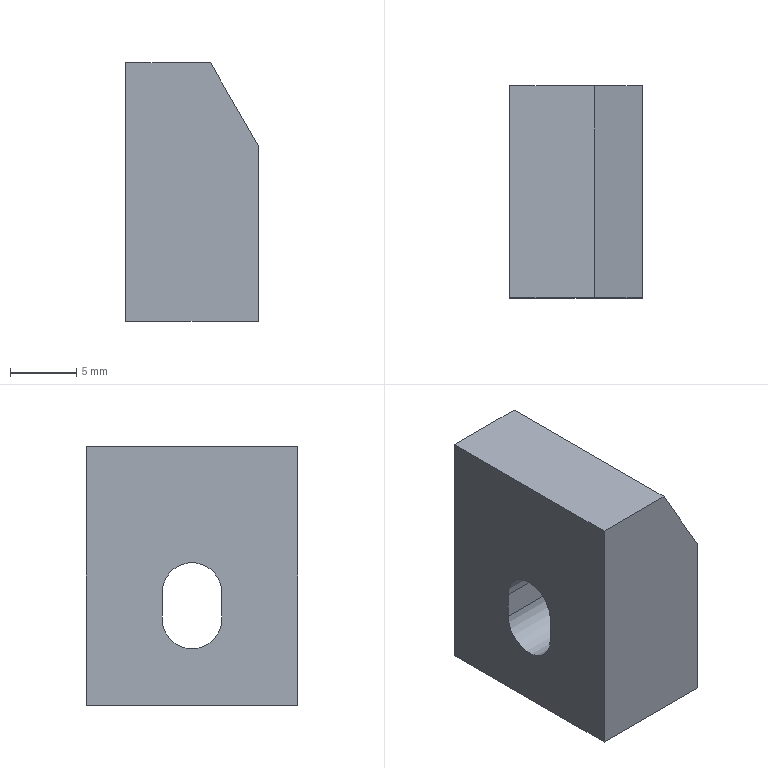Part | STEP file | 4-20.sldasm-Part-196 | 1 solid | 16 faces | box 10 x 16 x 19.5 mm | volume 2443 mm3 | plane 12 | cylinder 4 | commonest cylinder face diameters 4.5 x2 8 x2
STEP:
#1=CARTESIAN_POINT('',(132.065,605.425,-80.993));
#2=VERTEX_POINT('',#1);
#3=CARTESIAN_POINT('',(132.065,605.425,-100.493));
#4=VERTEX_POINT('',#3);
#5=CARTESIAN_POINT('',(132.065,605.425,-73.493));
#6=DIRECTION('',(0.,0.,-1.));
#7=VECTOR('',#6,1000.);
#8=LINE('',#5,#7);
#9=EDGE_CURVE('',#2,#4,#8,.T.);
#10=ORIENTED_EDGE('',*,*,#9,.T.);
#11=CARTESIAN_POINT('',(132.065,589.425,-100.493));
#12=VERTEX_POINT('',#11);
#13=CARTESIAN_POINT('',(132.065,589.425,-100.493));
#14=DIRECTION('',(0.,1.,0.));
#15=VECTOR('',#14,1000.);
#16=LINE('',#13,#15);
#17=EDGE_CURVE('',#12,#4,#16,.T.);
#18=ORIENTED_EDGE('',*,*,#17,.F.);
#19=CARTESIAN_POINT('',(132.065,589.425,-80.993));
#20=VERTEX_POINT('',#19);
#21=CARTESIAN_POINT('',(132.065,589.425,-73.493));
#22=DIRECTION('',(0.,0.,-1.));
#23=VECTOR('',#22,1000.);
#24=LINE('',#21,#23);
#25=EDGE_CURVE('',#20,#12,#24,.T.);
#26=ORIENTED_EDGE('',*,*,#25,.F.);
#27=CARTESIAN_POINT('',(132.065,1166.425,-80.993));
#28=DIRECTION('',(0.,1.,0.));
#29=VECTOR('',#28,1000.);
#30=LINE('',#27,#29);
#31=EDGE_CURVE('',#20,#2,#30,.T.);
#32=ORIENTED_EDGE('',*,*,#31,.T.);
#33=EDGE_LOOP('',(#10,#18,#26,#32));
#34=FACE_OUTER_BOUND('',#33,.T.);
#35=CARTESIAN_POINT('',(132.065,599.675,-93.993));
#36=VERTEX_POINT('',#35);
#37=CARTESIAN_POINT('',(132.065,595.175,-93.993));
#38=VERTEX_POINT('',#37);
#39=CARTESIAN_POINT('',(132.065,597.425,-93.993));
#40=DIRECTION('',(-1.,0.,0.));
#41=DIRECTION('',(0.,-1.,0.));
#42=AXIS2_PLACEMENT_3D('',#39,#40,#41);
#43=CIRCLE('',#42,2.25);
#44=EDGE_CURVE('',#36,#38,#43,.T.);
#45=ORIENTED_EDGE('',*,*,#44,.F.);
#46=CARTESIAN_POINT('',(132.065,599.675,-91.993));
#47=VERTEX_POINT('',#46);
#48=CARTESIAN_POINT('',(132.065,599.675,-73.493));
#49=DIRECTION('',(0.,0.,1.));
#50=VECTOR('',#49,1000.);
#51=LINE('',#48,#50);
#52=EDGE_CURVE('',#36,#47,#51,.T.);
#53=ORIENTED_EDGE('',*,*,#52,.T.);
#54=CARTESIAN_POINT('',(132.065,595.175,-91.993));
#55=VERTEX_POINT('',#54);
#56=CARTESIAN_POINT('',(132.065,597.425,-91.993));
#57=DIRECTION('',(-1.,0.,0.));
#58=DIRECTION('',(0.,-1.,0.));
#59=AXIS2_PLACEMENT_3D('',#56,#57,#58);
#60=CIRCLE('',#59,2.25);
#61=EDGE_CURVE('',#55,#47,#60,.T.);
#62=ORIENTED_EDGE('',*,*,#61,.F.);
#63=CARTESIAN_POINT('',(132.065,595.175,-73.493));
#64=DIRECTION('',(0.,0.,-1.));
#65=VECTOR('',#64,1000.);
#66=LINE('',#63,#65);
#67=EDGE_CURVE('',#55,#38,#66,.T.);
#68=ORIENTED_EDGE('',*,*,#67,.T.);
#69=EDGE_LOOP('',(#45,#53,#62,#68));
#70=FACE_BOUND('',#69,.T.);
#71=CARTESIAN_POINT('',(132.065,589.425,-73.493));
#72=DIRECTION('',(1.,0.,0.));
#73=DIRECTION('',(0.,-1.,0.));
#74=AXIS2_PLACEMENT_3D('',#71,#72,#73);
#75=PLANE('',#74);
#76=ADVANCED_FACE('',(#34,#70),#75,.F.);
#77=CARTESIAN_POINT('',(136.065,593.425,-93.993));
#78=VERTEX_POINT('',#77);
#79=CARTESIAN_POINT('',(136.065,601.425,-93.993));
#80=VERTEX_POINT('',#79);
#81=CARTESIAN_POINT('',(136.065,597.425,-93.993));
#82=DIRECTION('',(1.,0.,0.));
#83=DIRECTION('',(0.,-1.,0.));
#84=AXIS2_PLACEMENT_3D('',#81,#82,#83);
#85=CIRCLE('',#84,4.);
#86=EDGE_CURVE('',#78,#80,#85,.T.);
#87=ORIENTED_EDGE('',*,*,#86,.T.);
#88=CARTESIAN_POINT('',(136.065,601.425,-91.993));
#89=VERTEX_POINT('',#88);
#90=CARTESIAN_POINT('',(136.065,601.425,-97.993));
#91=DIRECTION('',(0.,0.,1.));
#92=VECTOR('',#91,1000.);
#93=LINE('',#90,#92);
#94=EDGE_CURVE('',#80,#89,#93,.T.);
#95=ORIENTED_EDGE('',*,*,#94,.T.);
#96=CARTESIAN_POINT('',(136.065,593.425,-91.993));
#97=VERTEX_POINT('',#96);
#98=CARTESIAN_POINT('',(136.065,597.425,-91.993));
#99=DIRECTION('',(1.,0.,0.));
#100=DIRECTION('',(0.,-1.,0.));
#101=AXIS2_PLACEMENT_3D('',#98,#99,#100);
#102=CIRCLE('',#101,4.);
#103=EDGE_CURVE('',#89,#97,#102,.T.);
#104=ORIENTED_EDGE('',*,*,#103,.T.);
#105=CARTESIAN_POINT('',(136.065,593.425,-97.993));
#106=DIRECTION('',(0.,0.,1.));
#107=VECTOR('',#106,1000.);
#108=LINE('',#105,#107);
#109=EDGE_CURVE('',#78,#97,#108,.T.);
#110=ORIENTED_EDGE('',*,*,#109,.F.);
#111=EDGE_LOOP('',(#87,#95,#104,#110));
#112=FACE_OUTER_BOUND('',#111,.T.);
#113=CARTESIAN_POINT('',(136.065,599.675,-93.993));
#114=VERTEX_POINT('',#113);
#115=CARTESIAN_POINT('',(136.065,599.675,-91.993));
#116=VERTEX_POINT('',#115);
#117=CARTESIAN_POINT('',(136.065,599.675,-97.993));
#118=DIRECTION('',(0.,0.,1.));
#119=VECTOR('',#118,1000.);
#120=LINE('',#117,#119);
#121=EDGE_CURVE('',#114,#116,#120,.T.);
#122=ORIENTED_EDGE('',*,*,#121,.F.);
#123=CARTESIAN_POINT('',(136.065,595.175,-93.993));
#124=VERTEX_POINT('',#123);
#125=CARTESIAN_POINT('',(136.065,597.425,-93.993));
#126=DIRECTION('',(-1.,0.,0.));
#127=DIRECTION('',(0.,-1.,0.));
#128=AXIS2_PLACEMENT_3D('',#125,#126,#127);
#129=CIRCLE('',#128,2.25);
#130=EDGE_CURVE('',#114,#124,#129,.T.);
#131=ORIENTED_EDGE('',*,*,#130,.T.);
#132=CARTESIAN_POINT('',(136.065,595.175,-91.993));
#133=VERTEX_POINT('',#132);
#134=CARTESIAN_POINT('',(136.065,595.175,-97.993));
#135=DIRECTION('',(0.,0.,-1.));
#136=VECTOR('',#135,1000.);
#137=LINE('',#134,#136);
#138=EDGE_CURVE('',#133,#124,#137,.T.);
#139=ORIENTED_EDGE('',*,*,#138,.F.);
#140=CARTESIAN_POINT('',(136.065,597.425,-91.993));
#141=DIRECTION('',(-1.,0.,0.));
#142=DIRECTION('',(0.,-1.,0.));
#143=AXIS2_PLACEMENT_3D('',#140,#141,#142);
#144=CIRCLE('',#143,2.25);
#145=EDGE_CURVE('',#133,#116,#144,.T.);
#146=ORIENTED_EDGE('',*,*,#145,.T.);
#147=EDGE_LOOP('',(#122,#131,#139,#146));
#148=FACE_BOUND('',#147,.T.);
#149=CARTESIAN_POINT('',(136.065,597.425,-97.993));
#150=DIRECTION('',(1.,0.,0.));
#151=DIRECTION('',(0.,-1.,0.));
#152=AXIS2_PLACEMENT_3D('',#149,#150,#151);
#153=PLANE('',#152);
#154=ADVANCED_FACE('',(#112,#148),#153,.T.);
#155=CARTESIAN_POINT('',(142.065,605.425,-100.493));
#156=VERTEX_POINT('',#155);
#157=CARTESIAN_POINT('',(142.065,605.425,-87.23));
#158=VERTEX_POINT('',#157);
#159=CARTESIAN_POINT('',(142.065,605.425,-103.493));
#160=DIRECTION('',(0.,0.,1.));
#161=VECTOR('',#160,1000.);
#162=LINE('',#159,#161);
#163=EDGE_CURVE('',#156,#158,#162,.T.);
#164=ORIENTED_EDGE('',*,*,#163,.T.);
#165=CARTESIAN_POINT('',(142.065,589.425,-87.23));
#166=VERTEX_POINT('',#165);
#167=CARTESIAN_POINT('',(142.065,605.425,-87.23));
#168=DIRECTION('',(0.,1.,0.));
#169=VECTOR('',#168,1000.);
#170=LINE('',#167,#169);
#171=EDGE_CURVE('',#166,#158,#170,.T.);
#172=ORIENTED_EDGE('',*,*,#171,.F.);
#173=CARTESIAN_POINT('',(142.065,589.425,-100.493));
#174=VERTEX_POINT('',#173);
#175=CARTESIAN_POINT('',(142.065,589.425,-103.493));
#176=DIRECTION('',(0.,0.,1.));
#177=VECTOR('',#176,1000.);
#178=LINE('',#175,#177);
#179=EDGE_CURVE('',#174,#166,#178,.T.);
#180=ORIENTED_EDGE('',*,*,#179,.F.);
#181=CARTESIAN_POINT('',(142.065,1211.425,-100.493));
#182=DIRECTION('',(0.,1.,0.));
#183=VECTOR('',#182,1000.);
#184=LINE('',#181,#183);
#185=EDGE_CURVE('',#174,#156,#184,.T.);
#186=ORIENTED_EDGE('',*,*,#185,.T.);
#187=EDGE_LOOP('',(#164,#172,#180,#186));
#188=FACE_OUTER_BOUND('',#187,.T.);
#189=CARTESIAN_POINT('',(142.065,593.425,-93.993));
#190=VERTEX_POINT('',#189);
#191=CARTESIAN_POINT('',(142.065,601.425,-93.993));
#192=VERTEX_POINT('',#191);
#193=CARTESIAN_POINT('',(142.065,597.425,-93.993));
#194=DIRECTION('',(1.,0.,0.));
#195=DIRECTION('',(0.,0.,-1.));
#196=AXIS2_PLACEMENT_3D('',#193,#194,#195);
#197=CIRCLE('',#196,4.);
#198=EDGE_CURVE('',#190,#192,#197,.T.);
#199=ORIENTED_EDGE('',*,*,#198,.F.);
#200=CARTESIAN_POINT('',(142.065,593.425,-91.993));
#201=VERTEX_POINT('',#200);
#202=CARTESIAN_POINT('',(142.065,593.425,-103.493));
#203=DIRECTION('',(0.,0.,1.));
#204=VECTOR('',#203,1000.);
#205=LINE('',#202,#204);
#206=EDGE_CURVE('',#190,#201,#205,.T.);
#207=ORIENTED_EDGE('',*,*,#206,.T.);
#208=CARTESIAN_POINT('',(142.065,601.425,-91.993));
#209=VERTEX_POINT('',#208);
#210=CARTESIAN_POINT('',(142.065,597.425,-91.993));
#211=DIRECTION('',(1.,0.,0.));
#212=DIRECTION('',(0.,0.,-1.));
#213=AXIS2_PLACEMENT_3D('',#210,#211,#212);
#214=CIRCLE('',#213,4.);
#215=EDGE_CURVE('',#209,#201,#214,.T.);
#216=ORIENTED_EDGE('',*,*,#215,.F.);
#217=CARTESIAN_POINT('',(142.065,601.425,-103.493));
#218=DIRECTION('',(0.,0.,1.));
#219=VECTOR('',#218,1000.);
#220=LINE('',#217,#219);
#221=EDGE_CURVE('',#192,#209,#220,.T.);
#222=ORIENTED_EDGE('',*,*,#221,.F.);
#223=EDGE_LOOP('',(#199,#207,#216,#222));
#224=FACE_BOUND('',#223,.T.);
#225=CARTESIAN_POINT('',(142.065,589.425,-103.493));
#226=DIRECTION('',(-1.,0.,0.));
#227=DIRECTION('',(0.,0.,-1.));
#228=AXIS2_PLACEMENT_3D('',#225,#226,#227);
#229=PLANE('',#228);
#230=ADVANCED_FACE('',(#188,#224),#229,.F.);
#231=CARTESIAN_POINT('',(132.065,605.425,-100.493));
#232=DIRECTION('',(1.,0.,0.));
#233=VECTOR('',#232,1000.);
#234=LINE('',#231,#233);
#235=EDGE_CURVE('',#4,#156,#234,.T.);
#236=ORIENTED_EDGE('',*,*,#235,.T.);
#237=ORIENTED_EDGE('',*,*,#185,.F.);
#238=CARTESIAN_POINT('',(132.065,589.425,-100.493));
#239=DIRECTION('',(1.,0.,0.));
#240=VECTOR('',#239,1000.);
#241=LINE('',#238,#240);
#242=EDGE_CURVE('',#12,#174,#241,.T.);
#243=ORIENTED_EDGE('',*,*,#242,.F.);
#244=ORIENTED_EDGE('',*,*,#17,.T.);
#245=EDGE_LOOP('',(#236,#237,#243,#244));
#246=FACE_OUTER_BOUND('',#245,.T.);
#247=CARTESIAN_POINT('',(-227.636,1211.425,-100.493));
#248=DIRECTION('',(0.,0.,-1.));
#249=DIRECTION('',(1.,0.,0.));
#250=AXIS2_PLACEMENT_3D('',#247,#248,#249);
#251=PLANE('',#250);
#252=ADVANCED_FACE('',(#246),#251,.T.);
#253=CARTESIAN_POINT('',(138.464,605.425,-80.993));
#254=VERTEX_POINT('',#253);
#255=CARTESIAN_POINT('',(142.065,605.425,-87.23));
#256=DIRECTION('',(-0.5,0.,0.866));
#257=VECTOR('',#256,1000.);
#258=LINE('',#255,#257);
#259=EDGE_CURVE('',#158,#254,#258,.T.);
#260=ORIENTED_EDGE('',*,*,#259,.T.);
#261=CARTESIAN_POINT('',(138.464,589.425,-80.993));
#262=VERTEX_POINT('',#261);
#263=CARTESIAN_POINT('',(138.464,605.425,-80.993));
#264=DIRECTION('',(0.,1.,0.));
#265=VECTOR('',#264,1000.);
#266=LINE('',#263,#265);
#267=EDGE_CURVE('',#262,#254,#266,.T.);
#268=ORIENTED_EDGE('',*,*,#267,.F.);
#269=CARTESIAN_POINT('',(142.065,589.425,-87.23));
#270=DIRECTION('',(-0.5,0.,0.866));
#271=VECTOR('',#270,1000.);
#272=LINE('',#269,#271);
#273=EDGE_CURVE('',#166,#262,#272,.T.);
#274=ORIENTED_EDGE('',*,*,#273,.F.);
#275=ORIENTED_EDGE('',*,*,#171,.T.);
#276=EDGE_LOOP('',(#260,#268,#274,#275));
#277=FACE_OUTER_BOUND('',#276,.T.);
#278=CARTESIAN_POINT('',(142.065,605.425,-87.23));
#279=DIRECTION('',(0.866,0.,0.5));
#280=DIRECTION('',(0.5,0.,-0.866));
#281=AXIS2_PLACEMENT_3D('',#278,#279,#280);
#282=PLANE('',#281);
#283=ADVANCED_FACE('',(#277),#282,.T.);
#284=CARTESIAN_POINT('',(132.065,605.425,-80.993));
#285=DIRECTION('',(-1.,0.,0.));
#286=VECTOR('',#285,1000.);
#287=LINE('',#284,#286);
#288=EDGE_CURVE('',#254,#2,#287,.T.);
#289=ORIENTED_EDGE('',*,*,#288,.T.);
#290=ORIENTED_EDGE('',*,*,#31,.F.);
#291=CARTESIAN_POINT('',(132.065,589.425,-80.993));
#292=DIRECTION('',(-1.,0.,0.));
#293=VECTOR('',#292,1000.);
#294=LINE('',#291,#293);
#295=EDGE_CURVE('',#262,#20,#294,.T.);
#296=ORIENTED_EDGE('',*,*,#295,.F.);
#297=ORIENTED_EDGE('',*,*,#267,.T.);
#298=EDGE_LOOP('',(#289,#290,#296,#297));
#299=FACE_OUTER_BOUND('',#298,.T.);
#300=CARTESIAN_POINT('',(152.993,1166.425,-80.993));
#301=DIRECTION('',(0.,0.,-1.));
#302=DIRECTION('',(-1.,0.,0.));
#303=AXIS2_PLACEMENT_3D('',#300,#301,#302);
#304=PLANE('',#303);
#305=ADVANCED_FACE('',(#299),#304,.F.);
#306=ORIENTED_EDGE('',*,*,#25,.T.);
#307=ORIENTED_EDGE('',*,*,#242,.T.);
#308=ORIENTED_EDGE('',*,*,#179,.T.);
#309=ORIENTED_EDGE('',*,*,#273,.T.);
#310=ORIENTED_EDGE('',*,*,#295,.T.);
#311=EDGE_LOOP('',(#306,#307,#308,#309,#310));
#312=FACE_OUTER_BOUND('',#311,.T.);
#313=CARTESIAN_POINT('',(132.065,589.425,-103.493));
#314=DIRECTION('',(0.,-1.,0.));
#315=DIRECTION('',(-1.,0.,0.));
#316=AXIS2_PLACEMENT_3D('',#313,#314,#315);
#317=PLANE('',#316);
#318=ADVANCED_FACE('',(#312),#317,.T.);
#319=ORIENTED_EDGE('',*,*,#9,.F.);
#320=ORIENTED_EDGE('',*,*,#288,.F.);
#321=ORIENTED_EDGE('',*,*,#259,.F.);
#322=ORIENTED_EDGE('',*,*,#163,.F.);
#323=ORIENTED_EDGE('',*,*,#235,.F.);
#324=EDGE_LOOP('',(#319,#320,#321,#322,#323));
#325=FACE_OUTER_BOUND('',#324,.T.);
#326=CARTESIAN_POINT('',(132.065,605.425,-103.493));
#327=DIRECTION('',(0.,-1.,0.));
#328=DIRECTION('',(-1.,0.,0.));
#329=AXIS2_PLACEMENT_3D('',#326,#327,#328);
#330=PLANE('',#329);
#331=ADVANCED_FACE('',(#325),#330,.F.);
#332=ORIENTED_EDGE('',*,*,#198,.T.);
#333=CARTESIAN_POINT('',(145.065,601.425,-93.993));
#334=DIRECTION('',(-1.,0.,0.));
#335=VECTOR('',#334,1000.);
#336=LINE('',#333,#335);
#337=EDGE_CURVE('',#192,#80,#336,.T.);
#338=ORIENTED_EDGE('',*,*,#337,.T.);
#339=ORIENTED_EDGE('',*,*,#86,.F.);
#340=CARTESIAN_POINT('',(145.065,593.425,-93.993));
#341=DIRECTION('',(-1.,0.,0.));
#342=VECTOR('',#341,1000.);
#343=LINE('',#340,#342);
#344=EDGE_CURVE('',#190,#78,#343,.T.);
#345=ORIENTED_EDGE('',*,*,#344,.F.);
#346=EDGE_LOOP('',(#332,#338,#339,#345));
#347=FACE_OUTER_BOUND('',#346,.T.);
#348=CARTESIAN_POINT('',(145.065,597.425,-93.993));
#349=DIRECTION('',(-1.,0.,0.));
#350=DIRECTION('',(0.,1.,0.));
#351=AXIS2_PLACEMENT_3D('',#348,#349,#350);
#352=CYLINDRICAL_SURFACE('',#351,4.);
#353=ADVANCED_FACE('',(#347),#352,.F.);
#354=ORIENTED_EDGE('',*,*,#221,.T.);
#355=CARTESIAN_POINT('',(145.065,601.425,-91.993));
#356=DIRECTION('',(-1.,0.,0.));
#357=VECTOR('',#356,1000.);
#358=LINE('',#355,#357);
#359=EDGE_CURVE('',#209,#89,#358,.T.);
#360=ORIENTED_EDGE('',*,*,#359,.T.);
#361=ORIENTED_EDGE('',*,*,#94,.F.);
#362=ORIENTED_EDGE('',*,*,#337,.F.);
#363=EDGE_LOOP('',(#354,#360,#361,#362));
#364=FACE_OUTER_BOUND('',#363,.T.);
#365=CARTESIAN_POINT('',(145.065,601.425,-97.993));
#366=DIRECTION('',(0.,-1.,0.));
#367=DIRECTION('',(-1.,0.,0.));
#368=AXIS2_PLACEMENT_3D('',#365,#366,#367);
#369=PLANE('',#368);
#370=ADVANCED_FACE('',(#364),#369,.T.);
#371=ORIENTED_EDGE('',*,*,#215,.T.);
#372=CARTESIAN_POINT('',(145.065,593.425,-91.993));
#373=DIRECTION('',(-1.,0.,0.));
#374=VECTOR('',#373,1000.);
#375=LINE('',#372,#374);
#376=EDGE_CURVE('',#201,#97,#375,.T.);
#377=ORIENTED_EDGE('',*,*,#376,.T.);
#378=ORIENTED_EDGE('',*,*,#103,.F.);
#379=ORIENTED_EDGE('',*,*,#359,.F.);
#380=EDGE_LOOP('',(#371,#377,#378,#379));
#381=FACE_OUTER_BOUND('',#380,.T.);
#382=CARTESIAN_POINT('',(145.065,597.425,-91.993));
#383=DIRECTION('',(-1.,0.,0.));
#384=DIRECTION('',(0.,1.,0.));
#385=AXIS2_PLACEMENT_3D('',#382,#383,#384);
#386=CYLINDRICAL_SURFACE('',#385,4.);
#387=ADVANCED_FACE('',(#381),#386,.F.);
#388=ORIENTED_EDGE('',*,*,#344,.T.);
#389=ORIENTED_EDGE('',*,*,#109,.T.);
#390=ORIENTED_EDGE('',*,*,#376,.F.);
#391=ORIENTED_EDGE('',*,*,#206,.F.);
#392=EDGE_LOOP('',(#388,#389,#390,#391));
#393=FACE_OUTER_BOUND('',#392,.T.);
#394=CARTESIAN_POINT('',(145.065,593.425,-97.993));
#395=DIRECTION('',(0.,-1.,0.));
#396=DIRECTION('',(-1.,0.,0.));
#397=AXIS2_PLACEMENT_3D('',#394,#395,#396);
#398=PLANE('',#397);
#399=ADVANCED_FACE('',(#393),#398,.F.);
#400=ORIENTED_EDGE('',*,*,#44,.T.);
#401=CARTESIAN_POINT('',(145.065,595.175,-93.993));
#402=DIRECTION('',(-1.,0.,0.));
#403=VECTOR('',#402,1000.);
#404=LINE('',#401,#403);
#405=EDGE_CURVE('',#124,#38,#404,.T.);
#406=ORIENTED_EDGE('',*,*,#405,.F.);
#407=ORIENTED_EDGE('',*,*,#130,.F.);
#408=CARTESIAN_POINT('',(145.065,599.675,-93.993));
#409=DIRECTION('',(-1.,0.,0.));
#410=VECTOR('',#409,1000.);
#411=LINE('',#408,#410);
#412=EDGE_CURVE('',#114,#36,#411,.T.);
#413=ORIENTED_EDGE('',*,*,#412,.T.);
#414=EDGE_LOOP('',(#400,#406,#407,#413));
#415=FACE_OUTER_BOUND('',#414,.T.);
#416=CARTESIAN_POINT('',(145.065,597.425,-93.993));
#417=DIRECTION('',(-1.,0.,0.));
#418=DIRECTION('',(0.,1.,0.));
#419=AXIS2_PLACEMENT_3D('',#416,#417,#418);
#420=CYLINDRICAL_SURFACE('',#419,2.25);
#421=ADVANCED_FACE('',(#415),#420,.F.);
#422=ORIENTED_EDGE('',*,*,#412,.F.);
#423=ORIENTED_EDGE('',*,*,#121,.T.);
#424=CARTESIAN_POINT('',(145.065,599.675,-91.993));
#425=DIRECTION('',(-1.,0.,0.));
#426=VECTOR('',#425,1000.);
#427=LINE('',#424,#426);
#428=EDGE_CURVE('',#116,#47,#427,.T.);
#429=ORIENTED_EDGE('',*,*,#428,.T.);
#430=ORIENTED_EDGE('',*,*,#52,.F.);
#431=EDGE_LOOP('',(#422,#423,#429,#430));
#432=FACE_OUTER_BOUND('',#431,.T.);
#433=CARTESIAN_POINT('',(145.065,599.675,-91.993));
#434=DIRECTION('',(0.,1.,0.));
#435=DIRECTION('',(0.,0.,-1.));
#436=AXIS2_PLACEMENT_3D('',#433,#434,#435);
#437=PLANE('',#436);
#438=ADVANCED_FACE('',(#432),#437,.F.);
#439=ORIENTED_EDGE('',*,*,#61,.T.);
#440=ORIENTED_EDGE('',*,*,#428,.F.);
#441=ORIENTED_EDGE('',*,*,#145,.F.);
#442=CARTESIAN_POINT('',(145.065,595.175,-91.993));
#443=DIRECTION('',(-1.,0.,0.));
#444=VECTOR('',#443,1000.);
#445=LINE('',#442,#444);
#446=EDGE_CURVE('',#133,#55,#445,.T.);
#447=ORIENTED_EDGE('',*,*,#446,.T.);
#448=EDGE_LOOP('',(#439,#440,#441,#447));
#449=FACE_OUTER_BOUND('',#448,.T.);
#450=CARTESIAN_POINT('',(145.065,597.425,-91.993));
#451=DIRECTION('',(-1.,0.,0.));
#452=DIRECTION('',(0.,1.,0.));
#453=AXIS2_PLACEMENT_3D('',#450,#451,#452);
#454=CYLINDRICAL_SURFACE('',#453,2.25);
#455=ADVANCED_FACE('',(#449),#454,.F.);
#456=ORIENTED_EDGE('',*,*,#446,.F.);
#457=ORIENTED_EDGE('',*,*,#138,.T.);
#458=ORIENTED_EDGE('',*,*,#405,.T.);
#459=ORIENTED_EDGE('',*,*,#67,.F.);
#460=EDGE_LOOP('',(#456,#457,#458,#459));
#461=FACE_OUTER_BOUND('',#460,.T.);
#462=CARTESIAN_POINT('',(145.065,595.175,-97.993));
#463=DIRECTION('',(0.,-1.,0.));
#464=DIRECTION('',(0.,0.,1.));
#465=AXIS2_PLACEMENT_3D('',#462,#463,#464);
#466=PLANE('',#465);
#467=ADVANCED_FACE('',(#461),#466,.F.);
#468=CLOSED_SHELL('',(#76,#154,#230,#252,#283,#305,#318,#331,#353,#370,#387,#399,#421,#438,#455,#467));
#469=MANIFOLD_SOLID_BREP('',#468);
#470=CARTESIAN_POINT('',(0.,0.,0.));
#471=DIRECTION('',(0.,0.,1.));
#472=DIRECTION('',(1.,0.,0.));
#473=AXIS2_PLACEMENT_3D('',#470,#471,#472);
#474=(LENGTH_UNIT()NAMED_UNIT(*)SI_UNIT(.MILLI.,.METRE.));
#475=UNCERTAINTY_MEASURE_WITH_UNIT(LENGTH_MEASURE(0.00001),#474,'','');
#476=(NAMED_UNIT(*)PLANE_ANGLE_UNIT()SI_UNIT($,.RADIAN.));
#477=(NAMED_UNIT(*)SI_UNIT($,.STERADIAN.)SOLID_ANGLE_UNIT());
#478=(GEOMETRIC_REPRESENTATION_CONTEXT(3)GLOBAL_UNCERTAINTY_ASSIGNED_CONTEXT((#475))GLOBAL_UNIT_ASSIGNED_CONTEXT((#474,#476,#477))REPRESENTATION_CONTEXT('',''));
#479=ADVANCED_BREP_SHAPE_REPRESENTATION('',(#469,#473),#478);